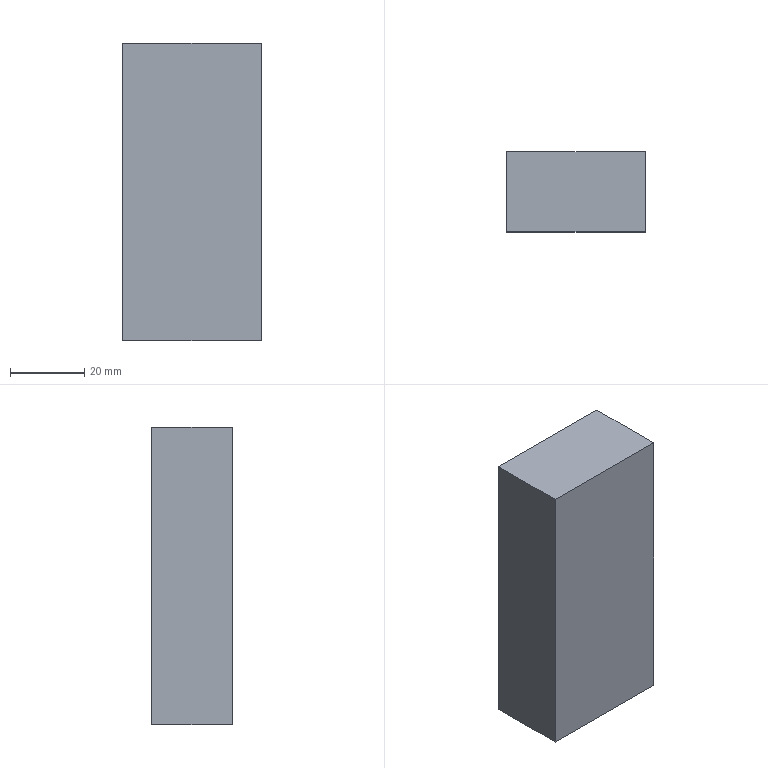Part | STEP file | Part 8^出料机械手-2 | 1 solid | 6 faces | box 37.433 x 21.616 x 80 mm | volume 64732 mm3 | plane 6
STEP:
#1=CARTESIAN_POINT('',(68.717,-10.808,0.));
#2=VERTEX_POINT('',#1);
#3=CARTESIAN_POINT('',(68.717,10.808,0.));
#4=VERTEX_POINT('',#3);
#5=CARTESIAN_POINT('',(68.717,-10.808,0.));
#6=DIRECTION('',(0.,1.,0.));
#7=VECTOR('',#6,1000.);
#8=LINE('',#5,#7);
#9=EDGE_CURVE('',#2,#4,#8,.T.);
#10=ORIENTED_EDGE('',*,*,#9,.T.);
#11=CARTESIAN_POINT('',(68.717,10.808,80.));
#12=VERTEX_POINT('',#11);
#13=CARTESIAN_POINT('',(68.717,10.808,80.));
#14=DIRECTION('',(0.,0.,-1.));
#15=VECTOR('',#14,1000.);
#16=LINE('',#13,#15);
#17=EDGE_CURVE('',#12,#4,#16,.T.);
#18=ORIENTED_EDGE('',*,*,#17,.F.);
#19=CARTESIAN_POINT('',(68.717,-10.808,80.));
#20=VERTEX_POINT('',#19);
#21=CARTESIAN_POINT('',(68.717,-10.808,80.));
#22=DIRECTION('',(0.,1.,0.));
#23=VECTOR('',#22,1000.);
#24=LINE('',#21,#23);
#25=EDGE_CURVE('',#20,#12,#24,.T.);
#26=ORIENTED_EDGE('',*,*,#25,.F.);
#27=CARTESIAN_POINT('',(68.717,-10.808,80.));
#28=DIRECTION('',(0.,0.,-1.));
#29=VECTOR('',#28,1000.);
#30=LINE('',#27,#29);
#31=EDGE_CURVE('',#20,#2,#30,.T.);
#32=ORIENTED_EDGE('',*,*,#31,.T.);
#33=EDGE_LOOP('',(#10,#18,#26,#32));
#34=FACE_OUTER_BOUND('',#33,.T.);
#35=CARTESIAN_POINT('',(68.717,-10.808,80.));
#36=DIRECTION('',(-1.,0.,0.));
#37=DIRECTION('',(0.,0.,1.));
#38=AXIS2_PLACEMENT_3D('',#35,#36,#37);
#39=PLANE('',#38);
#40=ADVANCED_FACE('',(#34),#39,.F.);
#41=CARTESIAN_POINT('',(31.283,10.808,0.));
#42=VERTEX_POINT('',#41);
#43=CARTESIAN_POINT('',(31.283,10.808,0.));
#44=DIRECTION('',(-1.,0.,0.));
#45=VECTOR('',#44,1000.);
#46=LINE('',#43,#45);
#47=EDGE_CURVE('',#4,#42,#46,.T.);
#48=ORIENTED_EDGE('',*,*,#47,.T.);
#49=CARTESIAN_POINT('',(31.283,10.808,80.));
#50=VERTEX_POINT('',#49);
#51=CARTESIAN_POINT('',(31.283,10.808,80.));
#52=DIRECTION('',(0.,0.,-1.));
#53=VECTOR('',#52,1000.);
#54=LINE('',#51,#53);
#55=EDGE_CURVE('',#50,#42,#54,.T.);
#56=ORIENTED_EDGE('',*,*,#55,.F.);
#57=CARTESIAN_POINT('',(31.283,10.808,80.));
#58=DIRECTION('',(-1.,0.,0.));
#59=VECTOR('',#58,1000.);
#60=LINE('',#57,#59);
#61=EDGE_CURVE('',#12,#50,#60,.T.);
#62=ORIENTED_EDGE('',*,*,#61,.F.);
#63=ORIENTED_EDGE('',*,*,#17,.T.);
#64=EDGE_LOOP('',(#48,#56,#62,#63));
#65=FACE_OUTER_BOUND('',#64,.T.);
#66=CARTESIAN_POINT('',(31.283,10.808,80.));
#67=DIRECTION('',(0.,-1.,0.));
#68=DIRECTION('',(0.,0.,-1.));
#69=AXIS2_PLACEMENT_3D('',#66,#67,#68);
#70=PLANE('',#69);
#71=ADVANCED_FACE('',(#65),#70,.F.);
#72=CARTESIAN_POINT('',(31.283,-10.808,0.));
#73=VERTEX_POINT('',#72);
#74=CARTESIAN_POINT('',(31.283,-10.808,0.));
#75=DIRECTION('',(0.,-1.,0.));
#76=VECTOR('',#75,1000.);
#77=LINE('',#74,#76);
#78=EDGE_CURVE('',#42,#73,#77,.T.);
#79=ORIENTED_EDGE('',*,*,#78,.T.);
#80=CARTESIAN_POINT('',(31.283,-10.808,80.));
#81=VERTEX_POINT('',#80);
#82=CARTESIAN_POINT('',(31.283,-10.808,80.));
#83=DIRECTION('',(0.,0.,-1.));
#84=VECTOR('',#83,1000.);
#85=LINE('',#82,#84);
#86=EDGE_CURVE('',#81,#73,#85,.T.);
#87=ORIENTED_EDGE('',*,*,#86,.F.);
#88=CARTESIAN_POINT('',(31.283,-10.808,80.));
#89=DIRECTION('',(0.,-1.,0.));
#90=VECTOR('',#89,1000.);
#91=LINE('',#88,#90);
#92=EDGE_CURVE('',#50,#81,#91,.T.);
#93=ORIENTED_EDGE('',*,*,#92,.F.);
#94=ORIENTED_EDGE('',*,*,#55,.T.);
#95=EDGE_LOOP('',(#79,#87,#93,#94));
#96=FACE_OUTER_BOUND('',#95,.T.);
#97=CARTESIAN_POINT('',(31.283,-10.808,80.));
#98=DIRECTION('',(1.,0.,0.));
#99=DIRECTION('',(0.,0.,-1.));
#100=AXIS2_PLACEMENT_3D('',#97,#98,#99);
#101=PLANE('',#100);
#102=ADVANCED_FACE('',(#96),#101,.F.);
#103=CARTESIAN_POINT('',(31.283,-10.808,0.));
#104=DIRECTION('',(1.,0.,0.));
#105=VECTOR('',#104,1000.);
#106=LINE('',#103,#105);
#107=EDGE_CURVE('',#73,#2,#106,.T.);
#108=ORIENTED_EDGE('',*,*,#107,.T.);
#109=ORIENTED_EDGE('',*,*,#31,.F.);
#110=CARTESIAN_POINT('',(31.283,-10.808,80.));
#111=DIRECTION('',(1.,0.,0.));
#112=VECTOR('',#111,1000.);
#113=LINE('',#110,#112);
#114=EDGE_CURVE('',#81,#20,#113,.T.);
#115=ORIENTED_EDGE('',*,*,#114,.F.);
#116=ORIENTED_EDGE('',*,*,#86,.T.);
#117=EDGE_LOOP('',(#108,#109,#115,#116));
#118=FACE_OUTER_BOUND('',#117,.T.);
#119=CARTESIAN_POINT('',(31.283,-10.808,80.));
#120=DIRECTION('',(0.,1.,0.));
#121=DIRECTION('',(0.,0.,1.));
#122=AXIS2_PLACEMENT_3D('',#119,#120,#121);
#123=PLANE('',#122);
#124=ADVANCED_FACE('',(#118),#123,.F.);
#125=ORIENTED_EDGE('',*,*,#25,.T.);
#126=ORIENTED_EDGE('',*,*,#61,.T.);
#127=ORIENTED_EDGE('',*,*,#92,.T.);
#128=ORIENTED_EDGE('',*,*,#114,.T.);
#129=EDGE_LOOP('',(#125,#126,#127,#128));
#130=FACE_OUTER_BOUND('',#129,.T.);
#131=CARTESIAN_POINT('',(68.717,10.808,80.));
#132=DIRECTION('',(0.,0.,-1.));
#133=DIRECTION('',(-1.,0.,0.));
#134=AXIS2_PLACEMENT_3D('',#131,#132,#133);
#135=PLANE('',#134);
#136=ADVANCED_FACE('',(#130),#135,.F.);
#137=ORIENTED_EDGE('',*,*,#9,.F.);
#138=ORIENTED_EDGE('',*,*,#107,.F.);
#139=ORIENTED_EDGE('',*,*,#78,.F.);
#140=ORIENTED_EDGE('',*,*,#47,.F.);
#141=EDGE_LOOP('',(#137,#138,#139,#140));
#142=FACE_OUTER_BOUND('',#141,.T.);
#143=CARTESIAN_POINT('',(68.717,10.808,0.));
#144=DIRECTION('',(0.,0.,-1.));
#145=DIRECTION('',(-1.,0.,0.));
#146=AXIS2_PLACEMENT_3D('',#143,#144,#145);
#147=PLANE('',#146);
#148=ADVANCED_FACE('',(#142),#147,.T.);
#149=CLOSED_SHELL('',(#40,#71,#102,#124,#136,#148));
#150=MANIFOLD_SOLID_BREP('',#149);
#151=CARTESIAN_POINT('',(0.,0.,0.));
#152=DIRECTION('',(0.,0.,1.));
#153=DIRECTION('',(1.,0.,0.));
#154=AXIS2_PLACEMENT_3D('',#151,#152,#153);
#155=(LENGTH_UNIT()NAMED_UNIT(*)SI_UNIT(.MILLI.,.METRE.));
#156=UNCERTAINTY_MEASURE_WITH_UNIT(LENGTH_MEASURE(0.00001),#155,'','');
#157=(NAMED_UNIT(*)PLANE_ANGLE_UNIT()SI_UNIT($,.RADIAN.));
#158=(NAMED_UNIT(*)SI_UNIT($,.STERADIAN.)SOLID_ANGLE_UNIT());
#159=(GEOMETRIC_REPRESENTATION_CONTEXT(3)GLOBAL_UNCERTAINTY_ASSIGNED_CONTEXT((#156))GLOBAL_UNIT_ASSIGNED_CONTEXT((#155,#157,#158))REPRESENTATION_CONTEXT('',''));
#160=ADVANCED_BREP_SHAPE_REPRESENTATION('',(#150,#154),#159);